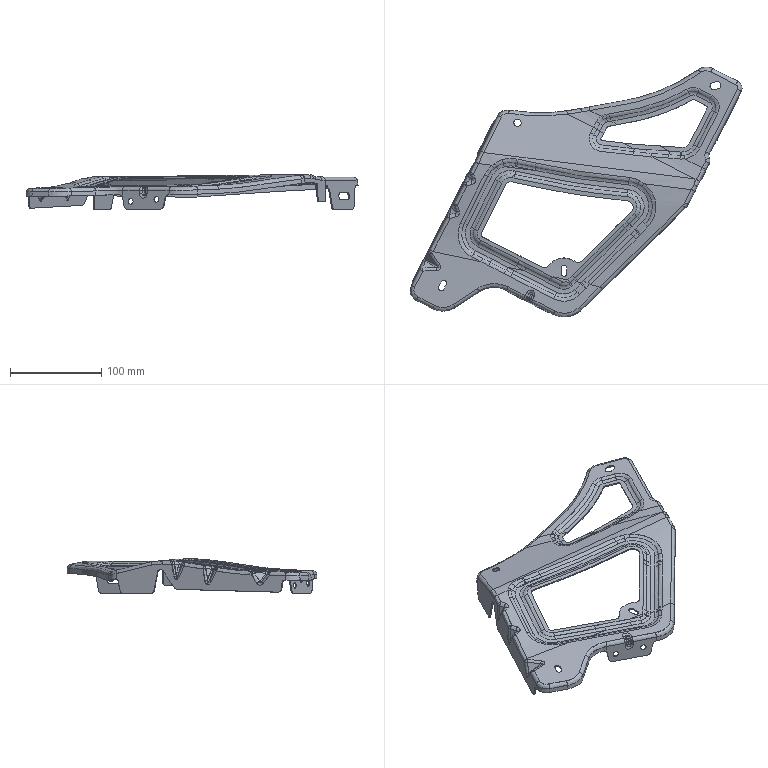Part | STEP file | 9805823280.1BPIECE_SOLIDE_FINALE_id854_x_t | 1 solid | 615 faces | box 364.643 x 274.564 x 38.362 mm | volume 69005 mm3 | spline 420 | cylinder 86 | plane 71 | other 18 | sphere 16 | torus 4 | commonest cylinder face diameters 5.5 x22 8 x19 6.2 x8 8.2 x7 3 x4 4.5 x4